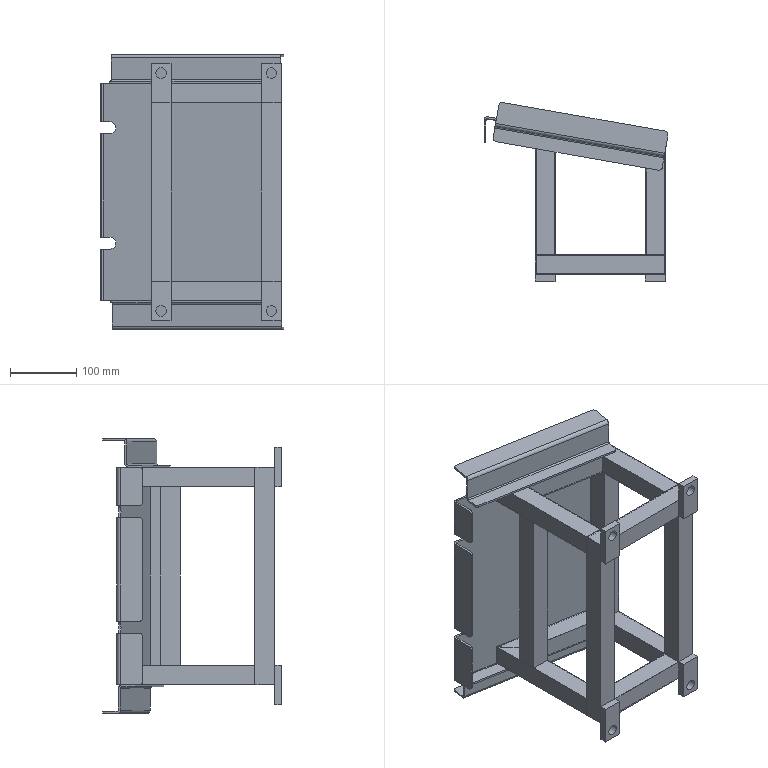Part | NX | features guide rail pipe2_Default_As Machined_ 20 | 19 solids | 218 faces | box 278.549 x 270.487 x 416 mm | volume 850854 mm3 | plane 182 | cylinder 36 | commonest cylinder face diameters 10 x23 4 x7 16 x4 18 x2